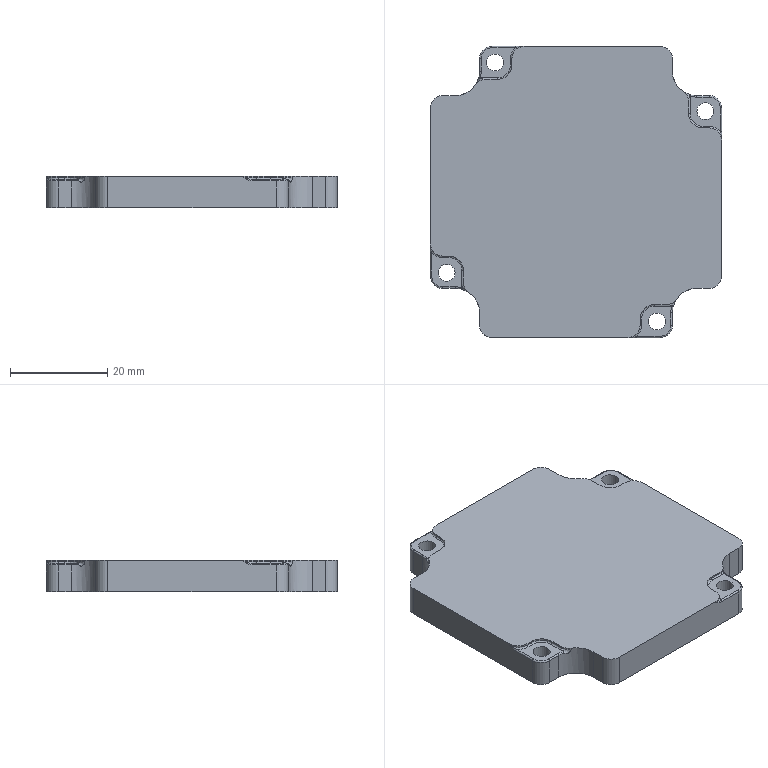Part | STEP file | 1 solid | 98 faces | box 60 x 60 x 6.4 mm | volume 20143 mm3 | cylinder 44 | plane 26 | torus 16 | spline 12 | commonest cylinder face diameters 0.6 x16 5 x16 3.5 x4 6 x4 10 x4